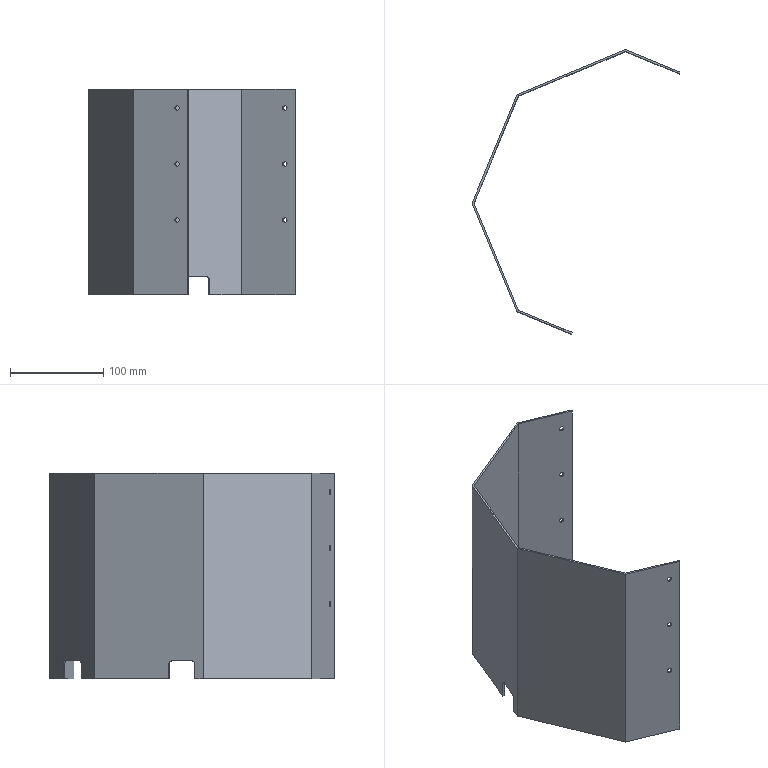Part | SolidWorks | features Cut 2, Fillet 2, ICE 2, Extrusion 1, RefAxis 1, Shell 1 | 1 solid | 38 faces | box 222.691 x 304.953 x 220 mm | volume 216770 mm3 | plane 22 | cylinder 16 | commonest cylinder face diameters 5 x12 10 x4
STEP:
#1=CARTESIAN_POINT('',(-66.179,-134.946,80.));
#2=VERTEX_POINT('',#1);
#3=CARTESIAN_POINT('',(-70.799,-133.033,80.));
#4=VERTEX_POINT('',#3);
#5=CARTESIAN_POINT('',(-68.489,-133.99,80.));
#6=DIRECTION('',(0.3827,0.9239,0.));
#7=DIRECTION('',(-0.9239,0.3827,0.));
#8=AXIS2_PLACEMENT_3D('',#5,#6,#7);
#9=CIRCLE('',#8,2.5);
#10=EDGE_CURVE('',#2,#4,#9,.T.);
#11=ORIENTED_EDGE('',*,*,#10,.T.);
#12=CARTESIAN_POINT('',(-71.564,-134.881,80.));
#13=VERTEX_POINT('',#12);
#14=CARTESIAN_POINT('',(53.29,166.544,80.));
#15=DIRECTION('',(-0.3827,-0.9239,0.));
#16=VECTOR('',#15,1000.);
#17=LINE('',#14,#16);
#18=EDGE_CURVE('',#4,#13,#17,.T.);
#19=ORIENTED_EDGE('',*,*,#18,.T.);
#20=CARTESIAN_POINT('',(-66.945,-136.794,80.));
#21=VERTEX_POINT('',#20);
#22=CARTESIAN_POINT('',(-69.254,-135.837,80.));
#23=DIRECTION('',(-0.3827,-0.9239,0.));
#24=DIRECTION('',(0.9239,-0.3827,0.));
#25=AXIS2_PLACEMENT_3D('',#22,#23,#24);
#26=CIRCLE('',#25,2.5);
#27=EDGE_CURVE('',#13,#21,#26,.T.);
#28=ORIENTED_EDGE('',*,*,#27,.T.);
#29=CARTESIAN_POINT('',(57.91,164.631,80.));
#30=DIRECTION('',(-0.3827,-0.9239,0.));
#31=VECTOR('',#30,1000.);
#32=LINE('',#29,#31);
#33=EDGE_CURVE('',#2,#21,#32,.T.);
#34=ORIENTED_EDGE('',*,*,#33,.F.);
#35=EDGE_LOOP('',(#11,#19,#28,#34));
#36=FACE_OUTER_BOUND('',#35,.T.);
#37=CARTESIAN_POINT('',(55.6,165.587,80.));
#38=DIRECTION('',(-0.3827,-0.9239,0.));
#39=DIRECTION('',(0.9239,-0.3827,0.));
#40=AXIS2_PLACEMENT_3D('',#37,#38,#39);
#41=CYLINDRICAL_SURFACE('',#40,2.5);
#42=ADVANCED_FACE('',(#36),#41,.F.);
#43=CARTESIAN_POINT('',(44.772,145.979,80.));
#44=VERTEX_POINT('',#43);
#45=CARTESIAN_POINT('',(49.391,144.065,80.));
#46=VERTEX_POINT('',#45);
#47=CARTESIAN_POINT('',(47.081,145.022,80.));
#48=DIRECTION('',(-0.3827,-0.9239,0.));
#49=DIRECTION('',(0.9239,-0.3827,0.));
#50=AXIS2_PLACEMENT_3D('',#47,#48,#49);
#51=CIRCLE('',#50,2.5);
#52=EDGE_CURVE('',#44,#46,#51,.T.);
#53=ORIENTED_EDGE('',*,*,#52,.F.);
#54=CARTESIAN_POINT('',(44.006,144.131,80.));
#55=VERTEX_POINT('',#54);
#56=CARTESIAN_POINT('',(53.29,166.544,80.));
#57=DIRECTION('',(-0.3827,-0.9239,0.));
#58=VECTOR('',#57,1000.);
#59=LINE('',#56,#58);
#60=EDGE_CURVE('',#44,#55,#59,.T.);
#61=ORIENTED_EDGE('',*,*,#60,.T.);
#62=CARTESIAN_POINT('',(48.626,142.217,80.));
#63=VERTEX_POINT('',#62);
#64=CARTESIAN_POINT('',(46.316,143.174,80.));
#65=DIRECTION('',(-0.3827,-0.9239,0.));
#66=DIRECTION('',(0.9239,-0.3827,0.));
#67=AXIS2_PLACEMENT_3D('',#64,#65,#66);
#68=CIRCLE('',#67,2.5);
#69=EDGE_CURVE('',#55,#63,#68,.T.);
#70=ORIENTED_EDGE('',*,*,#69,.T.);
#71=CARTESIAN_POINT('',(57.91,164.631,80.));
#72=DIRECTION('',(-0.3827,-0.9239,0.));
#73=VECTOR('',#72,1000.);
#74=LINE('',#71,#73);
#75=EDGE_CURVE('',#46,#63,#74,.T.);
#76=ORIENTED_EDGE('',*,*,#75,.F.);
#77=EDGE_LOOP('',(#53,#61,#70,#76));
#78=FACE_OUTER_BOUND('',#77,.T.);
#79=CARTESIAN_POINT('',(55.6,165.587,80.));
#80=DIRECTION('',(-0.3827,-0.9239,0.));
#81=DIRECTION('',(0.9239,-0.3827,0.));
#82=AXIS2_PLACEMENT_3D('',#79,#80,#81);
#83=CYLINDRICAL_SURFACE('',#82,2.5);
#84=ADVANCED_FACE('',(#78),#83,.F.);
#85=CARTESIAN_POINT('',(-66.179,-134.946,140.));
#86=VERTEX_POINT('',#85);
#87=CARTESIAN_POINT('',(-70.799,-133.033,140.));
#88=VERTEX_POINT('',#87);
#89=CARTESIAN_POINT('',(-68.489,-133.99,140.));
#90=DIRECTION('',(0.3827,0.9239,0.));
#91=DIRECTION('',(-0.9239,0.3827,0.));
#92=AXIS2_PLACEMENT_3D('',#89,#90,#91);
#93=CIRCLE('',#92,2.5);
#94=EDGE_CURVE('',#86,#88,#93,.T.);
#95=ORIENTED_EDGE('',*,*,#94,.T.);
#96=CARTESIAN_POINT('',(-71.564,-134.881,140.));
#97=VERTEX_POINT('',#96);
#98=CARTESIAN_POINT('',(53.29,166.544,140.));
#99=DIRECTION('',(-0.3827,-0.9239,0.));
#100=VECTOR('',#99,1000.);
#101=LINE('',#98,#100);
#102=EDGE_CURVE('',#88,#97,#101,.T.);
#103=ORIENTED_EDGE('',*,*,#102,.T.);
#104=CARTESIAN_POINT('',(-66.945,-136.794,140.));
#105=VERTEX_POINT('',#104);
#106=CARTESIAN_POINT('',(-69.254,-135.837,140.));
#107=DIRECTION('',(-0.3827,-0.9239,0.));
#108=DIRECTION('',(0.9239,-0.3827,0.));
#109=AXIS2_PLACEMENT_3D('',#106,#107,#108);
#110=CIRCLE('',#109,2.5);
#111=EDGE_CURVE('',#97,#105,#110,.T.);
#112=ORIENTED_EDGE('',*,*,#111,.T.);
#113=CARTESIAN_POINT('',(57.91,164.631,140.));
#114=DIRECTION('',(-0.3827,-0.9239,0.));
#115=VECTOR('',#114,1000.);
#116=LINE('',#113,#115);
#117=EDGE_CURVE('',#86,#105,#116,.T.);
#118=ORIENTED_EDGE('',*,*,#117,.F.);
#119=EDGE_LOOP('',(#95,#103,#112,#118));
#120=FACE_OUTER_BOUND('',#119,.T.);
#121=CARTESIAN_POINT('',(55.6,165.587,140.));
#122=DIRECTION('',(-0.3827,-0.9239,0.));
#123=DIRECTION('',(0.9239,-0.3827,0.));
#124=AXIS2_PLACEMENT_3D('',#121,#122,#123);
#125=CYLINDRICAL_SURFACE('',#124,2.5);
#126=ADVANCED_FACE('',(#120),#125,.F.);
#127=CARTESIAN_POINT('',(44.772,145.979,140.));
#128=VERTEX_POINT('',#127);
#129=CARTESIAN_POINT('',(49.391,144.065,140.));
#130=VERTEX_POINT('',#129);
#131=CARTESIAN_POINT('',(47.081,145.022,140.));
#132=DIRECTION('',(-0.3827,-0.9239,0.));
#133=DIRECTION('',(0.9239,-0.3827,0.));
#134=AXIS2_PLACEMENT_3D('',#131,#132,#133);
#135=CIRCLE('',#134,2.5);
#136=EDGE_CURVE('',#128,#130,#135,.T.);
#137=ORIENTED_EDGE('',*,*,#136,.F.);
#138=CARTESIAN_POINT('',(44.006,144.131,140.));
#139=VERTEX_POINT('',#138);
#140=CARTESIAN_POINT('',(53.29,166.544,140.));
#141=DIRECTION('',(-0.3827,-0.9239,0.));
#142=VECTOR('',#141,1000.);
#143=LINE('',#140,#142);
#144=EDGE_CURVE('',#128,#139,#143,.T.);
#145=ORIENTED_EDGE('',*,*,#144,.T.);
#146=CARTESIAN_POINT('',(48.626,142.217,140.));
#147=VERTEX_POINT('',#146);
#148=CARTESIAN_POINT('',(46.316,143.174,140.));
#149=DIRECTION('',(-0.3827,-0.9239,0.));
#150=DIRECTION('',(0.9239,-0.3827,0.));
#151=AXIS2_PLACEMENT_3D('',#148,#149,#150);
#152=CIRCLE('',#151,2.5);
#153=EDGE_CURVE('',#139,#147,#152,.T.);
#154=ORIENTED_EDGE('',*,*,#153,.T.);
#155=CARTESIAN_POINT('',(57.91,164.631,140.));
#156=DIRECTION('',(-0.3827,-0.9239,0.));
#157=VECTOR('',#156,1000.);
#158=LINE('',#155,#157);
#159=EDGE_CURVE('',#130,#147,#158,.T.);
#160=ORIENTED_EDGE('',*,*,#159,.F.);
#161=EDGE_LOOP('',(#137,#145,#154,#160));
#162=FACE_OUTER_BOUND('',#161,.T.);
#163=CARTESIAN_POINT('',(55.6,165.587,140.));
#164=DIRECTION('',(-0.3827,-0.9239,0.));
#165=DIRECTION('',(0.9239,-0.3827,0.));
#166=AXIS2_PLACEMENT_3D('',#163,#164,#165);
#167=CYLINDRICAL_SURFACE('',#166,2.5);
#168=ADVANCED_FACE('',(#162),#167,.F.);
#169=CARTESIAN_POINT('',(-66.179,-134.946,200.));
#170=VERTEX_POINT('',#169);
#171=CARTESIAN_POINT('',(-70.799,-133.033,200.));
#172=VERTEX_POINT('',#171);
#173=CARTESIAN_POINT('',(-68.489,-133.99,200.));
#174=DIRECTION('',(0.3827,0.9239,0.));
#175=DIRECTION('',(-0.9239,0.3827,0.));
#176=AXIS2_PLACEMENT_3D('',#173,#174,#175);
#177=CIRCLE('',#176,2.5);
#178=EDGE_CURVE('',#170,#172,#177,.T.);
#179=ORIENTED_EDGE('',*,*,#178,.T.);
#180=CARTESIAN_POINT('',(-71.564,-134.881,200.));
#181=VERTEX_POINT('',#180);
#182=CARTESIAN_POINT('',(53.29,166.544,200.));
#183=DIRECTION('',(-0.3827,-0.9239,0.));
#184=VECTOR('',#183,1000.);
#185=LINE('',#182,#184);
#186=EDGE_CURVE('',#172,#181,#185,.T.);
#187=ORIENTED_EDGE('',*,*,#186,.T.);
#188=CARTESIAN_POINT('',(-66.945,-136.794,200.));
#189=VERTEX_POINT('',#188);
#190=CARTESIAN_POINT('',(-69.254,-135.837,200.));
#191=DIRECTION('',(-0.3827,-0.9239,0.));
#192=DIRECTION('',(0.9239,-0.3827,0.));
#193=AXIS2_PLACEMENT_3D('',#190,#191,#192);
#194=CIRCLE('',#193,2.5);
#195=EDGE_CURVE('',#181,#189,#194,.T.);
#196=ORIENTED_EDGE('',*,*,#195,.T.);
#197=CARTESIAN_POINT('',(57.91,164.631,200.));
#198=DIRECTION('',(-0.3827,-0.9239,0.));
#199=VECTOR('',#198,1000.);
#200=LINE('',#197,#199);
#201=EDGE_CURVE('',#170,#189,#200,.T.);
#202=ORIENTED_EDGE('',*,*,#201,.F.);
#203=EDGE_LOOP('',(#179,#187,#196,#202));
#204=FACE_OUTER_BOUND('',#203,.T.);
#205=CARTESIAN_POINT('',(55.6,165.587,200.));
#206=DIRECTION('',(-0.3827,-0.9239,0.));
#207=DIRECTION('',(0.9239,-0.3827,0.));
#208=AXIS2_PLACEMENT_3D('',#205,#206,#207);
#209=CYLINDRICAL_SURFACE('',#208,2.5);
#210=ADVANCED_FACE('',(#204),#209,.F.);
#211=CARTESIAN_POINT('',(44.772,145.979,200.));
#212=VERTEX_POINT('',#211);
#213=CARTESIAN_POINT('',(49.391,144.065,200.));
#214=VERTEX_POINT('',#213);
#215=CARTESIAN_POINT('',(47.081,145.022,200.));
#216=DIRECTION('',(-0.3827,-0.9239,0.));
#217=DIRECTION('',(0.9239,-0.3827,0.));
#218=AXIS2_PLACEMENT_3D('',#215,#216,#217);
#219=CIRCLE('',#218,2.5);
#220=EDGE_CURVE('',#212,#214,#219,.T.);
#221=ORIENTED_EDGE('',*,*,#220,.F.);
#222=CARTESIAN_POINT('',(44.006,144.131,200.));
#223=VERTEX_POINT('',#222);
#224=CARTESIAN_POINT('',(53.29,166.544,200.));
#225=DIRECTION('',(-0.3827,-0.9239,0.));
#226=VECTOR('',#225,1000.);
#227=LINE('',#224,#226);
#228=EDGE_CURVE('',#212,#223,#227,.T.);
#229=ORIENTED_EDGE('',*,*,#228,.T.);
#230=CARTESIAN_POINT('',(48.626,142.217,200.));
#231=VERTEX_POINT('',#230);
#232=CARTESIAN_POINT('',(46.316,143.174,200.));
#233=DIRECTION('',(-0.3827,-0.9239,0.));
#234=DIRECTION('',(0.9239,-0.3827,0.));
#235=AXIS2_PLACEMENT_3D('',#232,#233,#234);
#236=CIRCLE('',#235,2.5);
#237=EDGE_CURVE('',#223,#231,#236,.T.);
#238=ORIENTED_EDGE('',*,*,#237,.T.);
#239=CARTESIAN_POINT('',(57.91,164.631,200.));
#240=DIRECTION('',(-0.3827,-0.9239,0.));
#241=VECTOR('',#240,1000.);
#242=LINE('',#239,#241);
#243=EDGE_CURVE('',#214,#231,#242,.T.);
#244=ORIENTED_EDGE('',*,*,#243,.F.);
#245=EDGE_LOOP('',(#221,#229,#238,#244));
#246=FACE_OUTER_BOUND('',#245,.T.);
#247=CARTESIAN_POINT('',(55.6,165.587,200.));
#248=DIRECTION('',(-0.3827,-0.9239,0.));
#249=DIRECTION('',(0.9239,-0.3827,0.));
#250=AXIS2_PLACEMENT_3D('',#247,#248,#249);
#251=CYLINDRICAL_SURFACE('',#250,2.5);
#252=ADVANCED_FACE('',(#246),#251,.F.);
#253=CARTESIAN_POINT('',(0.,162.359,0.));
#254=VERTEX_POINT('',#253);
#255=CARTESIAN_POINT('',(-34.269,148.164,0.));
#256=VERTEX_POINT('',#255);
#257=CARTESIAN_POINT('',(0.7654,162.676,0.));
#258=DIRECTION('',(-0.9239,-0.3827,0.));
#259=VECTOR('',#258,1000.);
#260=LINE('',#257,#259);
#261=EDGE_CURVE('',#254,#256,#260,.T.);
#262=ORIENTED_EDGE('',*,*,#261,.T.);
#263=CARTESIAN_POINT('',(-35.034,150.012,0.));
#264=VERTEX_POINT('',#263);
#265=CARTESIAN_POINT('',(81.301,-130.847,0.));
#266=DIRECTION('',(-0.3827,0.9239,0.));
#267=VECTOR('',#266,1000.);
#268=LINE('',#265,#267);
#269=EDGE_CURVE('',#256,#264,#268,.T.);
#270=ORIENTED_EDGE('',*,*,#269,.T.);
#271=CARTESIAN_POINT('',(0.,164.524,0.));
#272=VERTEX_POINT('',#271);
#273=CARTESIAN_POINT('',(0.,164.524,0.));
#274=DIRECTION('',(-0.9239,-0.3827,0.));
#275=VECTOR('',#274,1000.);
#276=LINE('',#273,#275);
#277=EDGE_CURVE('',#272,#264,#276,.T.);
#278=ORIENTED_EDGE('',*,*,#277,.F.);
#279=CARTESIAN_POINT('',(58.168,140.43,0.));
#280=VERTEX_POINT('',#279);
#281=CARTESIAN_POINT('',(116.336,116.336,0.));
#282=DIRECTION('',(-0.9239,0.3827,0.));
#283=VECTOR('',#282,1000.);
#284=LINE('',#281,#283);
#285=EDGE_CURVE('',#280,#272,#284,.T.);
#286=ORIENTED_EDGE('',*,*,#285,.F.);
#287=CARTESIAN_POINT('',(57.403,138.582,0.));
#288=VERTEX_POINT('',#287);
#289=CARTESIAN_POINT('',(75.617,182.555,0.));
#290=DIRECTION('',(-0.3827,-0.9239,0.));
#291=VECTOR('',#290,1000.);
#292=LINE('',#289,#291);
#293=EDGE_CURVE('',#280,#288,#292,.T.);
#294=ORIENTED_EDGE('',*,*,#293,.T.);
#295=CARTESIAN_POINT('',(115.57,114.488,0.));
#296=DIRECTION('',(-0.9239,0.3827,0.));
#297=VECTOR('',#296,1000.);
#298=LINE('',#295,#297);
#299=EDGE_CURVE('',#288,#254,#298,.T.);
#300=ORIENTED_EDGE('',*,*,#299,.T.);
#301=EDGE_LOOP('',(#262,#270,#278,#286,#294,#300));
#302=FACE_OUTER_BOUND('',#301,.T.);
#303=CARTESIAN_POINT('',(0.,0.,0.));
#304=DIRECTION('',(0.,0.,1.));
#305=DIRECTION('',(1.,0.,0.));
#306=AXIS2_PLACEMENT_3D('',#303,#304,#305);
#307=PLANE('',#306);
#308=ADVANCED_FACE('',(#302),#307,.F.);
#309=CARTESIAN_POINT('',(-81.228,130.878,0.));
#310=VERTEX_POINT('',#309);
#311=CARTESIAN_POINT('',(-116.336,116.336,0.));
#312=VERTEX_POINT('',#311);
#313=CARTESIAN_POINT('',(0.,164.524,0.));
#314=DIRECTION('',(-0.9239,-0.3827,0.));
#315=VECTOR('',#314,1000.);
#316=LINE('',#313,#315);
#317=EDGE_CURVE('',#310,#312,#316,.T.);
#318=ORIENTED_EDGE('',*,*,#317,.F.);
#319=CARTESIAN_POINT('',(-80.463,129.03,0.));
#320=VERTEX_POINT('',#319);
#321=CARTESIAN_POINT('',(35.107,-149.982,0.));
#322=DIRECTION('',(-0.3827,0.9239,0.));
#323=VECTOR('',#322,1000.);
#324=LINE('',#321,#323);
#325=EDGE_CURVE('',#320,#310,#324,.T.);
#326=ORIENTED_EDGE('',*,*,#325,.F.);
#327=CARTESIAN_POINT('',(-114.805,114.805,0.));
#328=VERTEX_POINT('',#327);
#329=CARTESIAN_POINT('',(0.7654,162.676,0.));
#330=DIRECTION('',(-0.9239,-0.3827,0.));
#331=VECTOR('',#330,1000.);
#332=LINE('',#329,#331);
#333=EDGE_CURVE('',#320,#328,#332,.T.);
#334=ORIENTED_EDGE('',*,*,#333,.T.);
#335=CARTESIAN_POINT('',(-147.369,36.19,0.));
#336=VERTEX_POINT('',#335);
#337=CARTESIAN_POINT('',(-114.488,115.57,0.));
#338=DIRECTION('',(-0.3827,-0.9239,0.));
#339=VECTOR('',#338,1000.);
#340=LINE('',#337,#339);
#341=EDGE_CURVE('',#328,#336,#340,.T.);
#342=ORIENTED_EDGE('',*,*,#341,.T.);
#343=CARTESIAN_POINT('',(-149.216,36.955,0.));
#344=VERTEX_POINT('',#343);
#345=CARTESIAN_POINT('',(90.512,-62.344,0.));
#346=DIRECTION('',(-0.9239,0.3827,0.));
#347=VECTOR('',#346,1000.);
#348=LINE('',#345,#347);
#349=EDGE_CURVE('',#336,#344,#348,.T.);
#350=ORIENTED_EDGE('',*,*,#349,.T.);
#351=CARTESIAN_POINT('',(-116.336,116.336,0.));
#352=DIRECTION('',(-0.3827,-0.9239,0.));
#353=VECTOR('',#352,1000.);
#354=LINE('',#351,#353);
#355=EDGE_CURVE('',#312,#344,#354,.T.);
#356=ORIENTED_EDGE('',*,*,#355,.F.);
#357=EDGE_LOOP('',(#318,#326,#334,#342,#350,#356));
#358=FACE_OUTER_BOUND('',#357,.T.);
#359=CARTESIAN_POINT('',(0.,0.,0.));
#360=DIRECTION('',(0.,0.,1.));
#361=DIRECTION('',(1.,0.,0.));
#362=AXIS2_PLACEMENT_3D('',#359,#360,#361);
#363=PLANE('',#362);
#364=ADVANCED_FACE('',(#358),#363,.F.);
#365=CARTESIAN_POINT('',(-69.254,-135.837,80.));
#366=DIRECTION('',(-0.3827,-0.9239,0.));
#367=DIRECTION('',(0.9239,-0.3827,0.));
#368=AXIS2_PLACEMENT_3D('',#365,#366,#367);
#369=CIRCLE('',#368,2.5);
#370=EDGE_CURVE('',#21,#13,#369,.T.);
#371=ORIENTED_EDGE('',*,*,#370,.F.);
#372=ORIENTED_EDGE('',*,*,#27,.F.);
#373=EDGE_LOOP('',(#371,#372));
#374=FACE_BOUND('',#373,.T.);
#375=CARTESIAN_POINT('',(-69.254,-135.837,140.));
#376=DIRECTION('',(-0.3827,-0.9239,0.));
#377=DIRECTION('',(0.9239,-0.3827,0.));
#378=AXIS2_PLACEMENT_3D('',#375,#376,#377);
#379=CIRCLE('',#378,2.5);
#380=EDGE_CURVE('',#105,#97,#379,.T.);
#381=ORIENTED_EDGE('',*,*,#380,.F.);
#382=ORIENTED_EDGE('',*,*,#111,.F.);
#383=EDGE_LOOP('',(#381,#382));
#384=FACE_BOUND('',#383,.T.);
#385=CARTESIAN_POINT('',(-69.254,-135.837,200.));
#386=DIRECTION('',(-0.3827,-0.9239,0.));
#387=DIRECTION('',(0.9239,-0.3827,0.));
#388=AXIS2_PLACEMENT_3D('',#385,#386,#387);
#389=CIRCLE('',#388,2.5);
#390=EDGE_CURVE('',#189,#181,#389,.T.);
#391=ORIENTED_EDGE('',*,*,#390,.F.);
#392=ORIENTED_EDGE('',*,*,#195,.F.);
#393=EDGE_LOOP('',(#391,#392));
#394=FACE_BOUND('',#393,.T.);
#395=CARTESIAN_POINT('',(-116.336,-116.336,0.));
#396=VERTEX_POINT('',#395);
#397=CARTESIAN_POINT('',(-58.168,-140.43,0.));
#398=VERTEX_POINT('',#397);
#399=CARTESIAN_POINT('',(-116.336,-116.336,0.));
#400=DIRECTION('',(0.9239,-0.3827,0.));
#401=VECTOR('',#400,1000.);
#402=LINE('',#399,#401);
#403=EDGE_CURVE('',#396,#398,#402,.T.);
#404=ORIENTED_EDGE('',*,*,#403,.T.);
#405=CARTESIAN_POINT('',(-58.168,-140.43,220.));
#406=VERTEX_POINT('',#405);
#407=CARTESIAN_POINT('',(-58.168,-140.43,220.));
#408=DIRECTION('',(0.,0.,1.));
#409=VECTOR('',#408,1000.);
#410=LINE('',#407,#409);
#411=EDGE_CURVE('',#398,#406,#410,.T.);
#412=ORIENTED_EDGE('',*,*,#411,.T.);
#413=CARTESIAN_POINT('',(-116.336,-116.336,220.));
#414=VERTEX_POINT('',#413);
#415=CARTESIAN_POINT('',(-116.336,-116.336,220.));
#416=DIRECTION('',(0.9239,-0.3827,0.));
#417=VECTOR('',#416,1000.);
#418=LINE('',#415,#417);
#419=EDGE_CURVE('',#414,#406,#418,.T.);
#420=ORIENTED_EDGE('',*,*,#419,.F.);
#421=CARTESIAN_POINT('',(-116.336,-116.336,220.));
#422=DIRECTION('',(0.,0.,-1.));
#423=VECTOR('',#422,1000.);
#424=LINE('',#421,#423);
#425=EDGE_CURVE('',#414,#396,#424,.T.);
#426=ORIENTED_EDGE('',*,*,#425,.T.);
#427=EDGE_LOOP('',(#404,#412,#420,#426));
#428=FACE_OUTER_BOUND('',#427,.T.);
#429=CARTESIAN_POINT('',(-116.336,-116.336,220.));
#430=DIRECTION('',(0.3827,0.9239,0.));
#431=DIRECTION('',(-0.9239,0.3827,0.));
#432=AXIS2_PLACEMENT_3D('',#429,#430,#431);
#433=PLANE('',#432);
#434=ADVANCED_FACE('',(#374,#384,#394,#428),#433,.F.);
#435=CARTESIAN_POINT('',(47.081,145.022,80.));
#436=DIRECTION('',(-0.3827,-0.9239,0.));
#437=DIRECTION('',(0.9239,-0.3827,0.));
#438=AXIS2_PLACEMENT_3D('',#435,#436,#437);
#439=CIRCLE('',#438,2.5);
#440=EDGE_CURVE('',#46,#44,#439,.T.);
#441=ORIENTED_EDGE('',*,*,#440,.T.);
#442=ORIENTED_EDGE('',*,*,#52,.T.);
#443=EDGE_LOOP('',(#441,#442));
#444=FACE_BOUND('',#443,.T.);
#445=CARTESIAN_POINT('',(47.081,145.022,140.));
#446=DIRECTION('',(-0.3827,-0.9239,0.));
#447=DIRECTION('',(0.9239,-0.3827,0.));
#448=AXIS2_PLACEMENT_3D('',#445,#446,#447);
#449=CIRCLE('',#448,2.5);
#450=EDGE_CURVE('',#130,#128,#449,.T.);
#451=ORIENTED_EDGE('',*,*,#450,.T.);
#452=ORIENTED_EDGE('',*,*,#136,.T.);
#453=EDGE_LOOP('',(#451,#452));
#454=FACE_BOUND('',#453,.T.);
#455=CARTESIAN_POINT('',(47.081,145.022,200.));
#456=DIRECTION('',(-0.3827,-0.9239,0.));
#457=DIRECTION('',(0.9239,-0.3827,0.));
#458=AXIS2_PLACEMENT_3D('',#455,#456,#457);
#459=CIRCLE('',#458,2.5);
#460=EDGE_CURVE('',#214,#212,#459,.T.);
#461=ORIENTED_EDGE('',*,*,#460,.T.);
#462=ORIENTED_EDGE('',*,*,#220,.T.);
#463=EDGE_LOOP('',(#461,#462));
#464=FACE_BOUND('',#463,.T.);
#465=CARTESIAN_POINT('',(58.168,140.43,220.));
#466=VERTEX_POINT('',#465);
#467=CARTESIAN_POINT('',(0.,164.524,220.));
#468=VERTEX_POINT('',#467);
#469=CARTESIAN_POINT('',(116.336,116.336,220.));
#470=DIRECTION('',(-0.9239,0.3827,0.));
#471=VECTOR('',#470,1000.);
#472=LINE('',#469,#471);
#473=EDGE_CURVE('',#466,#468,#472,.T.);
#474=ORIENTED_EDGE('',*,*,#473,.F.);
#475=CARTESIAN_POINT('',(58.168,140.43,220.));
#476=DIRECTION('',(0.,0.,-1.));
#477=VECTOR('',#476,1000.);
#478=LINE('',#475,#477);
#479=EDGE_CURVE('',#466,#280,#478,.T.);
#480=ORIENTED_EDGE('',*,*,#479,.T.);
#481=ORIENTED_EDGE('',*,*,#285,.T.);
#482=CARTESIAN_POINT('',(0.,164.524,220.));
#483=DIRECTION('',(0.,0.,-1.));
#484=VECTOR('',#483,1000.);
#485=LINE('',#482,#484);
#486=EDGE_CURVE('',#468,#272,#485,.T.);
#487=ORIENTED_EDGE('',*,*,#486,.F.);
#488=EDGE_LOOP('',(#474,#480,#481,#487));
#489=FACE_OUTER_BOUND('',#488,.T.);
#490=CARTESIAN_POINT('',(116.336,116.336,220.));
#491=DIRECTION('',(-0.3827,-0.9239,0.));
#492=DIRECTION('',(0.9239,-0.3827,0.));
#493=AXIS2_PLACEMENT_3D('',#490,#491,#492);
#494=PLANE('',#493);
#495=ADVANCED_FACE('',(#444,#454,#464,#489),#494,.F.);
#496=ORIENTED_EDGE('',*,*,#277,.T.);
#497=CARTESIAN_POINT('',(-35.034,150.012,15.));
#498=VERTEX_POINT('',#497);
#499=CARTESIAN_POINT('',(-35.034,150.012,0.));
#500=DIRECTION('',(0.,0.,-1.));
#501=VECTOR('',#500,1000.);
#502=LINE('',#499,#501);
#503=EDGE_CURVE('',#498,#264,#502,.T.);
#504=ORIENTED_EDGE('',*,*,#503,.F.);
#505=CARTESIAN_POINT('',(-39.654,148.098,20.));
#506=VERTEX_POINT('',#505);
#507=CARTESIAN_POINT('',(-39.654,148.098,15.));
#508=DIRECTION('',(0.3827,-0.9239,0.));
#509=DIRECTION('',(0.9239,0.3827,0.));
#510=AXIS2_PLACEMENT_3D('',#507,#508,#509);
#511=CIRCLE('',#510,5.);
#512=EDGE_CURVE('',#498,#506,#511,.T.);
#513=ORIENTED_EDGE('',*,*,#512,.T.);
#514=CARTESIAN_POINT('',(-76.609,132.791,20.));
#515=VERTEX_POINT('',#514);
#516=CARTESIAN_POINT('',(-35.034,150.012,20.));
#517=DIRECTION('',(0.9239,0.3827,0.));
#518=VECTOR('',#517,1000.);
#519=LINE('',#516,#518);
#520=EDGE_CURVE('',#515,#506,#519,.T.);
#521=ORIENTED_EDGE('',*,*,#520,.F.);
#522=CARTESIAN_POINT('',(-81.228,130.878,15.));
#523=VERTEX_POINT('',#522);
#524=CARTESIAN_POINT('',(-76.609,132.791,15.));
#525=DIRECTION('',(0.3827,-0.9239,0.));
#526=DIRECTION('',(0.9239,0.3827,0.));
#527=AXIS2_PLACEMENT_3D('',#524,#525,#526);
#528=CIRCLE('',#527,5.);
#529=EDGE_CURVE('',#515,#523,#528,.T.);
#530=ORIENTED_EDGE('',*,*,#529,.T.);
#531=CARTESIAN_POINT('',(-81.228,130.878,0.));
#532=DIRECTION('',(0.,0.,1.));
#533=VECTOR('',#532,1000.);
#534=LINE('',#531,#533);
#535=EDGE_CURVE('',#310,#523,#534,.T.);
#536=ORIENTED_EDGE('',*,*,#535,.F.);
#537=ORIENTED_EDGE('',*,*,#317,.T.);
#538=CARTESIAN_POINT('',(-116.336,116.336,220.));
#539=VERTEX_POINT('',#538);
#540=CARTESIAN_POINT('',(-116.336,116.336,220.));
#541=DIRECTION('',(0.,0.,-1.));
#542=VECTOR('',#541,1000.);
#543=LINE('',#540,#542);
#544=EDGE_CURVE('',#539,#312,#543,.T.);
#545=ORIENTED_EDGE('',*,*,#544,.F.);
#546=CARTESIAN_POINT('',(0.,164.524,220.));
#547=DIRECTION('',(-0.9239,-0.3827,0.));
#548=VECTOR('',#547,1000.);
#549=LINE('',#546,#548);
#550=EDGE_CURVE('',#468,#539,#549,.T.);
#551=ORIENTED_EDGE('',*,*,#550,.F.);
#552=ORIENTED_EDGE('',*,*,#486,.T.);
#553=EDGE_LOOP('',(#496,#504,#513,#521,#530,#536,#537,#545,#551,#552));
#554=FACE_OUTER_BOUND('',#553,.T.);
#555=CARTESIAN_POINT('',(0.,164.524,220.));
#556=DIRECTION('',(0.3827,-0.9239,0.));
#557=DIRECTION('',(0.9239,0.3827,0.));
#558=AXIS2_PLACEMENT_3D('',#555,#556,#557);
#559=PLANE('',#558);
#560=ADVANCED_FACE('',(#554),#559,.F.);
#561=ORIENTED_EDGE('',*,*,#355,.T.);
#562=CARTESIAN_POINT('',(-149.216,36.955,15.));
#563=VERTEX_POINT('',#562);
#564=CARTESIAN_POINT('',(-149.216,36.955,0.));
#565=DIRECTION('',(0.,0.,-1.));
#566=VECTOR('',#565,1000.);
#567=LINE('',#564,#566);
#568=EDGE_CURVE('',#563,#344,#567,.T.);
#569=ORIENTED_EDGE('',*,*,#568,.F.);
#570=CARTESIAN_POINT('',(-151.13,32.336,20.));
#571=VERTEX_POINT('',#570);
#572=CARTESIAN_POINT('',(-151.13,32.336,15.));
#573=DIRECTION('',(0.9239,-0.3827,0.));
#574=DIRECTION('',(0.3827,0.9239,0.));
#575=AXIS2_PLACEMENT_3D('',#572,#573,#574);
#576=CIRCLE('',#575,5.);
#577=EDGE_CURVE('',#563,#571,#576,.T.);
#578=ORIENTED_EDGE('',*,*,#577,.T.);
#579=CARTESIAN_POINT('',(-158.783,13.858,20.));
#580=VERTEX_POINT('',#579);
#581=CARTESIAN_POINT('',(-149.216,36.955,20.));
#582=DIRECTION('',(0.3827,0.9239,0.));
#583=VECTOR('',#582,1000.);
#584=LINE('',#581,#583);
#585=EDGE_CURVE('',#580,#571,#584,.T.);
#586=ORIENTED_EDGE('',*,*,#585,.F.);
#587=CARTESIAN_POINT('',(-160.697,9.239,15.));
#588=VERTEX_POINT('',#587);
#589=CARTESIAN_POINT('',(-158.783,13.858,15.));
#590=DIRECTION('',(0.9239,-0.3827,0.));
#591=DIRECTION('',(0.3827,0.9239,0.));
#592=AXIS2_PLACEMENT_3D('',#589,#590,#591);
#593=CIRCLE('',#592,5.);
#594=EDGE_CURVE('',#580,#588,#593,.T.);
#595=ORIENTED_EDGE('',*,*,#594,.T.);
#596=CARTESIAN_POINT('',(-160.697,9.239,0.));
#597=VERTEX_POINT('',#596);
#598=CARTESIAN_POINT('',(-160.697,9.239,0.));
#599=DIRECTION('',(0.,0.,1.));
#600=VECTOR('',#599,1000.);
#601=LINE('',#598,#600);
#602=EDGE_CURVE('',#597,#588,#601,.T.);
#603=ORIENTED_EDGE('',*,*,#602,.F.);
#604=CARTESIAN_POINT('',(-164.524,0.,0.));
#605=VERTEX_POINT('',#604);
#606=CARTESIAN_POINT('',(-116.336,116.336,0.));
#607=DIRECTION('',(-0.3827,-0.9239,0.));
#608=VECTOR('',#607,1000.);
#609=LINE('',#606,#608);
#610=EDGE_CURVE('',#597,#605,#609,.T.);
#611=ORIENTED_EDGE('',*,*,#610,.T.);
#612=CARTESIAN_POINT('',(-164.524,0.,220.));
#613=VERTEX_POINT('',#612);
#614=CARTESIAN_POINT('',(-164.524,0.,220.));
#615=DIRECTION('',(0.,0.,-1.));
#616=VECTOR('',#615,1000.);
#617=LINE('',#614,#616);
#618=EDGE_CURVE('',#613,#605,#617,.T.);
#619=ORIENTED_EDGE('',*,*,#618,.F.);
#620=CARTESIAN_POINT('',(-116.336,116.336,220.));
#621=DIRECTION('',(-0.3827,-0.9239,0.));
#622=VECTOR('',#621,1000.);
#623=LINE('',#620,#622);
#624=EDGE_CURVE('',#539,#613,#623,.T.);
#625=ORIENTED_EDGE('',*,*,#624,.F.);
#626=ORIENTED_EDGE('',*,*,#544,.T.);
#627=EDGE_LOOP('',(#561,#569,#578,#586,#595,#603,#611,#619,#625,#626));
#628=FACE_OUTER_BOUND('',#627,.T.);
#629=CARTESIAN_POINT('',(-116.336,116.336,220.));
#630=DIRECTION('',(0.9239,-0.3827,0.));
#631=DIRECTION('',(0.3827,0.9239,0.));
#632=AXIS2_PLACEMENT_3D('',#629,#630,#631);
#633=PLANE('',#632);
#634=ADVANCED_FACE('',(#628),#633,.F.);
#635=CARTESIAN_POINT('',(-164.524,0.,0.));
#636=DIRECTION('',(0.3827,-0.9239,0.));
#637=VECTOR('',#636,1000.);
#638=LINE('',#635,#637);
#639=EDGE_CURVE('',#605,#396,#638,.T.);
#640=ORIENTED_EDGE('',*,*,#639,.T.);
#641=ORIENTED_EDGE('',*,*,#425,.F.);
#642=CARTESIAN_POINT('',(-164.524,0.,220.));
#643=DIRECTION('',(0.3827,-0.9239,0.));
#644=VECTOR('',#643,1000.);
#645=LINE('',#642,#644);
#646=EDGE_CURVE('',#613,#414,#645,.T.);
#647=ORIENTED_EDGE('',*,*,#646,.F.);
#648=ORIENTED_EDGE('',*,*,#618,.T.);
#649=EDGE_LOOP('',(#640,#641,#647,#648));
#650=FACE_OUTER_BOUND('',#649,.T.);
#651=CARTESIAN_POINT('',(-164.524,0.,220.));
#652=DIRECTION('',(0.9239,0.3827,0.));
#653=DIRECTION('',(-0.3827,0.9239,0.));
#654=AXIS2_PLACEMENT_3D('',#651,#652,#653);
#655=PLANE('',#654);
#656=ADVANCED_FACE('',(#650),#655,.F.);
#657=CARTESIAN_POINT('',(57.403,138.582,220.));
#658=VERTEX_POINT('',#657);
#659=CARTESIAN_POINT('',(75.617,182.555,220.));
#660=DIRECTION('',(-0.3827,-0.9239,0.));
#661=VECTOR('',#660,1000.);
#662=LINE('',#659,#661);
#663=EDGE_CURVE('',#466,#658,#662,.T.);
#664=ORIENTED_EDGE('',*,*,#663,.F.);
#665=ORIENTED_EDGE('',*,*,#473,.T.);
#666=ORIENTED_EDGE('',*,*,#550,.T.);
#667=ORIENTED_EDGE('',*,*,#624,.T.);
#668=ORIENTED_EDGE('',*,*,#646,.T.);
#669=ORIENTED_EDGE('',*,*,#419,.T.);
#670=CARTESIAN_POINT('',(-57.403,-138.582,220.));
#671=VERTEX_POINT('',#670);
#672=CARTESIAN_POINT('',(75.617,182.555,220.));
#673=DIRECTION('',(-0.3827,-0.9239,0.));
#674=VECTOR('',#673,1000.);
#675=LINE('',#672,#674);
#676=EDGE_CURVE('',#671,#406,#675,.T.);
#677=ORIENTED_EDGE('',*,*,#676,.F.);
#678=CARTESIAN_POINT('',(-114.805,-114.805,220.));
#679=VERTEX_POINT('',#678);
#680=CARTESIAN_POINT('',(-115.57,-114.488,220.));
#681=DIRECTION('',(0.9239,-0.3827,0.));
#682=VECTOR('',#681,1000.);
#683=LINE('',#680,#682);
#684=EDGE_CURVE('',#679,#671,#683,.T.);
#685=ORIENTED_EDGE('',*,*,#684,.F.);
#686=CARTESIAN_POINT('',(-162.359,0.,220.));
#687=VERTEX_POINT('',#686);
#688=CARTESIAN_POINT('',(-162.676,0.7654,220.));
#689=DIRECTION('',(0.3827,-0.9239,0.));
#690=VECTOR('',#689,1000.);
#691=LINE('',#688,#690);
#692=EDGE_CURVE('',#687,#679,#691,.T.);
#693=ORIENTED_EDGE('',*,*,#692,.F.);
#694=CARTESIAN_POINT('',(-114.805,114.805,220.));
#695=VERTEX_POINT('',#694);
#696=CARTESIAN_POINT('',(-114.488,115.57,220.));
#697=DIRECTION('',(-0.3827,-0.9239,0.));
#698=VECTOR('',#697,1000.);
#699=LINE('',#696,#698);
#700=EDGE_CURVE('',#695,#687,#699,.T.);
#701=ORIENTED_EDGE('',*,*,#700,.F.);
#702=CARTESIAN_POINT('',(0.,162.359,220.));
#703=VERTEX_POINT('',#702);
#704=CARTESIAN_POINT('',(0.7654,162.676,220.));
#705=DIRECTION('',(-0.9239,-0.3827,0.));
#706=VECTOR('',#705,1000.);
#707=LINE('',#704,#706);
#708=EDGE_CURVE('',#703,#695,#707,.T.);
#709=ORIENTED_EDGE('',*,*,#708,.F.);
#710=CARTESIAN_POINT('',(115.57,114.488,220.));
#711=DIRECTION('',(-0.9239,0.3827,0.));
#712=VECTOR('',#711,1000.);
#713=LINE('',#710,#712);
#714=EDGE_CURVE('',#658,#703,#713,.T.);
#715=ORIENTED_EDGE('',*,*,#714,.F.);
#716=EDGE_LOOP('',(#664,#665,#666,#667,#668,#669,#677,#685,#693,#701,#709,#715));
#717=FACE_OUTER_BOUND('',#716,.T.);
#718=CARTESIAN_POINT('',(0.,0.,220.));
#719=DIRECTION('',(0.,0.,1.));
#720=DIRECTION('',(1.,0.,0.));
#721=AXIS2_PLACEMENT_3D('',#718,#719,#720);
#722=PLANE('',#721);
#723=ADVANCED_FACE('',(#717),#722,.T.);
#724=ORIENTED_EDGE('',*,*,#610,.F.);
#725=CARTESIAN_POINT('',(-158.849,8.473,0.));
#726=VERTEX_POINT('',#725);
#727=CARTESIAN_POINT('',(79.032,-90.06,0.));
#728=DIRECTION('',(-0.9239,0.3827,0.));
#729=VECTOR('',#728,1000.);
#730=LINE('',#727,#729);
#731=EDGE_CURVE('',#726,#597,#730,.T.);
#732=ORIENTED_EDGE('',*,*,#731,.F.);
#733=CARTESIAN_POINT('',(-162.359,0.,0.));
#734=VERTEX_POINT('',#733);
#735=CARTESIAN_POINT('',(-114.488,115.57,0.));
#736=DIRECTION('',(-0.3827,-0.9239,0.));
#737=VECTOR('',#736,1000.);
#738=LINE('',#735,#737);
#739=EDGE_CURVE('',#726,#734,#738,.T.);
#740=ORIENTED_EDGE('',*,*,#739,.T.);
#741=CARTESIAN_POINT('',(-114.805,-114.805,0.));
#742=VERTEX_POINT('',#741);
#743=CARTESIAN_POINT('',(-162.676,0.7654,0.));
#744=DIRECTION('',(0.3827,-0.9239,0.));
#745=VECTOR('',#744,1000.);
#746=LINE('',#743,#745);
#747=EDGE_CURVE('',#734,#742,#746,.T.);
#748=ORIENTED_EDGE('',*,*,#747,.T.);
#749=CARTESIAN_POINT('',(-57.403,-138.582,0.));
#750=VERTEX_POINT('',#749);
#751=CARTESIAN_POINT('',(-115.57,-114.488,0.));
#752=DIRECTION('',(0.9239,-0.3827,0.));
#753=VECTOR('',#752,1000.);
#754=LINE('',#751,#753);
#755=EDGE_CURVE('',#742,#750,#754,.T.);
#756=ORIENTED_EDGE('',*,*,#755,.T.);
#757=CARTESIAN_POINT('',(75.617,182.555,0.));
#758=DIRECTION('',(-0.3827,-0.9239,0.));
#759=VECTOR('',#758,1000.);
#760=LINE('',#757,#759);
#761=EDGE_CURVE('',#750,#398,#760,.T.);
#762=ORIENTED_EDGE('',*,*,#761,.T.);
#763=ORIENTED_EDGE('',*,*,#403,.F.);
#764=ORIENTED_EDGE('',*,*,#639,.F.);
#765=EDGE_LOOP('',(#724,#732,#740,#748,#756,#762,#763,#764));
#766=FACE_OUTER_BOUND('',#765,.T.);
#767=CARTESIAN_POINT('',(0.,0.,0.));
#768=DIRECTION('',(0.,0.,1.));
#769=DIRECTION('',(1.,0.,0.));
#770=AXIS2_PLACEMENT_3D('',#767,#768,#769);
#771=PLANE('',#770);
#772=ADVANCED_FACE('',(#766),#771,.F.);
#773=ORIENTED_EDGE('',*,*,#10,.F.);
#774=CARTESIAN_POINT('',(-68.489,-133.99,80.));
#775=DIRECTION('',(0.3827,0.9239,0.));
#776=DIRECTION('',(-0.9239,0.3827,0.));
#777=AXIS2_PLACEMENT_3D('',#774,#775,#776);
#778=CIRCLE('',#777,2.5);
#779=EDGE_CURVE('',#4,#2,#778,.T.);
#780=ORIENTED_EDGE('',*,*,#779,.F.);
#781=EDGE_LOOP('',(#773,#780));
#782=FACE_BOUND('',#781,.T.);
#783=ORIENTED_EDGE('',*,*,#94,.F.);
#784=CARTESIAN_POINT('',(-68.489,-133.99,140.));
#785=DIRECTION('',(0.3827,0.9239,0.));
#786=DIRECTION('',(-0.9239,0.3827,0.));
#787=AXIS2_PLACEMENT_3D('',#784,#785,#786);
#788=CIRCLE('',#787,2.5);
#789=EDGE_CURVE('',#88,#86,#788,.T.);
#790=ORIENTED_EDGE('',*,*,#789,.F.);
#791=EDGE_LOOP('',(#783,#790));
#792=FACE_BOUND('',#791,.T.);
#793=ORIENTED_EDGE('',*,*,#178,.F.);
#794=CARTESIAN_POINT('',(-68.489,-133.99,200.));
#795=DIRECTION('',(0.3827,0.9239,0.));
#796=DIRECTION('',(-0.9239,0.3827,0.));
#797=AXIS2_PLACEMENT_3D('',#794,#795,#796);
#798=CIRCLE('',#797,2.5);
#799=EDGE_CURVE('',#172,#170,#798,.T.);
#800=ORIENTED_EDGE('',*,*,#799,.F.);
#801=EDGE_LOOP('',(#793,#800));
#802=FACE_BOUND('',#801,.T.);
#803=CARTESIAN_POINT('',(-57.403,-138.582,220.));
#804=DIRECTION('',(0.,0.,1.));
#805=VECTOR('',#804,1000.);
#806=LINE('',#803,#805);
#807=EDGE_CURVE('',#750,#671,#806,.T.);
#808=ORIENTED_EDGE('',*,*,#807,.F.);
#809=ORIENTED_EDGE('',*,*,#755,.F.);
#810=CARTESIAN_POINT('',(-114.805,-114.805,220.));
#811=DIRECTION('',(0.,0.,-1.));
#812=VECTOR('',#811,1000.);
#813=LINE('',#810,#812);
#814=EDGE_CURVE('',#679,#742,#813,.T.);
#815=ORIENTED_EDGE('',*,*,#814,.F.);
#816=ORIENTED_EDGE('',*,*,#684,.T.);
#817=EDGE_LOOP('',(#808,#809,#815,#816));
#818=FACE_OUTER_BOUND('',#817,.T.);
#819=CARTESIAN_POINT('',(-115.57,-114.488,220.));
#820=DIRECTION('',(0.3827,0.9239,0.));
#821=DIRECTION('',(-0.9239,0.3827,0.));
#822=AXIS2_PLACEMENT_3D('',#819,#820,#821);
#823=PLANE('',#822);
#824=ADVANCED_FACE('',(#782,#792,#802,#818),#823,.T.);
#825=CARTESIAN_POINT('',(46.316,143.174,80.));
#826=DIRECTION('',(-0.3827,-0.9239,0.));
#827=DIRECTION('',(0.9239,-0.3827,0.));
#828=AXIS2_PLACEMENT_3D('',#825,#826,#827);
#829=CIRCLE('',#828,2.5);
#830=EDGE_CURVE('',#63,#55,#829,.T.);
#831=ORIENTED_EDGE('',*,*,#830,.F.);
#832=ORIENTED_EDGE('',*,*,#69,.F.);
#833=EDGE_LOOP('',(#831,#832));
#834=FACE_BOUND('',#833,.T.);
#835=CARTESIAN_POINT('',(46.316,143.174,140.));
#836=DIRECTION('',(-0.3827,-0.9239,0.));
#837=DIRECTION('',(0.9239,-0.3827,0.));
#838=AXIS2_PLACEMENT_3D('',#835,#836,#837);
#839=CIRCLE('',#838,2.5);
#840=EDGE_CURVE('',#147,#139,#839,.T.);
#841=ORIENTED_EDGE('',*,*,#840,.F.);
#842=ORIENTED_EDGE('',*,*,#153,.F.);
#843=EDGE_LOOP('',(#841,#842));
#844=FACE_BOUND('',#843,.T.);
#845=CARTESIAN_POINT('',(46.316,143.174,200.));
#846=DIRECTION('',(-0.3827,-0.9239,0.));
#847=DIRECTION('',(0.9239,-0.3827,0.));
#848=AXIS2_PLACEMENT_3D('',#845,#846,#847);
#849=CIRCLE('',#848,2.5);
#850=EDGE_CURVE('',#231,#223,#849,.T.);
#851=ORIENTED_EDGE('',*,*,#850,.F.);
#852=ORIENTED_EDGE('',*,*,#237,.F.);
#853=EDGE_LOOP('',(#851,#852));
#854=FACE_BOUND('',#853,.T.);
#855=CARTESIAN_POINT('',(57.403,138.582,220.));
#856=DIRECTION('',(0.,0.,-1.));
#857=VECTOR('',#856,1000.);
#858=LINE('',#855,#857);
#859=EDGE_CURVE('',#658,#288,#858,.T.);
#860=ORIENTED_EDGE('',*,*,#859,.F.);
#861=ORIENTED_EDGE('',*,*,#714,.T.);
#862=CARTESIAN_POINT('',(0.,162.359,220.));
#863=DIRECTION('',(0.,0.,-1.));
#864=VECTOR('',#863,1000.);
#865=LINE('',#862,#864);
#866=EDGE_CURVE('',#703,#254,#865,.T.);
#867=ORIENTED_EDGE('',*,*,#866,.T.);
#868=ORIENTED_EDGE('',*,*,#299,.F.);
#869=EDGE_LOOP('',(#860,#861,#867,#868));
#870=FACE_OUTER_BOUND('',#869,.T.);
#871=CARTESIAN_POINT('',(115.57,114.488,220.));
#872=DIRECTION('',(-0.3827,-0.9239,0.));
#873=DIRECTION('',(0.9239,-0.3827,0.));
#874=AXIS2_PLACEMENT_3D('',#871,#872,#873);
#875=PLANE('',#874);
#876=ADVANCED_FACE('',(#834,#844,#854,#870),#875,.T.);
#877=CARTESIAN_POINT('',(-34.269,148.164,15.));
#878=VERTEX_POINT('',#877);
#879=CARTESIAN_POINT('',(-34.269,148.164,220.));
#880=DIRECTION('',(0.,0.,1.));
#881=VECTOR('',#880,1000.);
#882=LINE('',#879,#881);
#883=EDGE_CURVE('',#256,#878,#882,.T.);
#884=ORIENTED_EDGE('',*,*,#883,.F.);
#885=ORIENTED_EDGE('',*,*,#261,.F.);
#886=ORIENTED_EDGE('',*,*,#866,.F.);
#887=ORIENTED_EDGE('',*,*,#708,.T.);
#888=CARTESIAN_POINT('',(-114.805,114.805,220.));
#889=DIRECTION('',(0.,0.,-1.));
#890=VECTOR('',#889,1000.);
#891=LINE('',#888,#890);
#892=EDGE_CURVE('',#695,#328,#891,.T.);
#893=ORIENTED_EDGE('',*,*,#892,.T.);
#894=ORIENTED_EDGE('',*,*,#333,.F.);
#895=CARTESIAN_POINT('',(-80.463,129.03,15.));
#896=VERTEX_POINT('',#895);
#897=CARTESIAN_POINT('',(-80.463,129.03,220.));
#898=DIRECTION('',(0.,0.,-1.));
#899=VECTOR('',#898,1000.);
#900=LINE('',#897,#899);
#901=EDGE_CURVE('',#896,#320,#900,.T.);
#902=ORIENTED_EDGE('',*,*,#901,.F.);
#903=CARTESIAN_POINT('',(-75.844,130.943,20.));
#904=VERTEX_POINT('',#903);
#905=CARTESIAN_POINT('',(-75.844,130.943,15.));
#906=DIRECTION('',(-0.3827,0.9239,0.));
#907=DIRECTION('',(0.9239,0.3827,0.));
#908=AXIS2_PLACEMENT_3D('',#905,#906,#907);
#909=CIRCLE('',#908,5.);
#910=EDGE_CURVE('',#896,#904,#909,.T.);
#911=ORIENTED_EDGE('',*,*,#910,.T.);
#912=CARTESIAN_POINT('',(-38.888,146.251,20.));
#913=VERTEX_POINT('',#912);
#914=CARTESIAN_POINT('',(0.7654,162.676,20.));
#915=DIRECTION('',(-0.9239,-0.3827,0.));
#916=VECTOR('',#915,1000.);
#917=LINE('',#914,#916);
#918=EDGE_CURVE('',#913,#904,#917,.T.);
#919=ORIENTED_EDGE('',*,*,#918,.F.);
#920=CARTESIAN_POINT('',(-38.888,146.251,15.));
#921=DIRECTION('',(-0.3827,0.9239,0.));
#922=DIRECTION('',(0.9239,0.3827,0.));
#923=AXIS2_PLACEMENT_3D('',#920,#921,#922);
#924=CIRCLE('',#923,5.);
#925=EDGE_CURVE('',#913,#878,#924,.T.);
#926=ORIENTED_EDGE('',*,*,#925,.T.);
#927=EDGE_LOOP('',(#884,#885,#886,#887,#893,#894,#902,#911,#919,#926));
#928=FACE_OUTER_BOUND('',#927,.T.);
#929=CARTESIAN_POINT('',(0.7654,162.676,220.));
#930=DIRECTION('',(0.3827,-0.9239,0.));
#931=DIRECTION('',(0.9239,0.3827,0.));
#932=AXIS2_PLACEMENT_3D('',#929,#930,#931);
#933=PLANE('',#932);
#934=ADVANCED_FACE('',(#928),#933,.T.);
#935=CARTESIAN_POINT('',(-147.369,36.19,15.));
#936=VERTEX_POINT('',#935);
#937=CARTESIAN_POINT('',(-147.369,36.19,220.));
#938=DIRECTION('',(0.,0.,1.));
#939=VECTOR('',#938,1000.);
#940=LINE('',#937,#939);
#941=EDGE_CURVE('',#336,#936,#940,.T.);
#942=ORIENTED_EDGE('',*,*,#941,.F.);
#943=ORIENTED_EDGE('',*,*,#341,.F.);
#944=ORIENTED_EDGE('',*,*,#892,.F.);
#945=ORIENTED_EDGE('',*,*,#700,.T.);
#946=CARTESIAN_POINT('',(-162.359,0.,220.));
#947=DIRECTION('',(0.,0.,-1.));
#948=VECTOR('',#947,1000.);
#949=LINE('',#946,#948);
#950=EDGE_CURVE('',#687,#734,#949,.T.);
#951=ORIENTED_EDGE('',*,*,#950,.T.);
#952=ORIENTED_EDGE('',*,*,#739,.F.);
#953=CARTESIAN_POINT('',(-158.849,8.473,15.));
#954=VERTEX_POINT('',#953);
#955=CARTESIAN_POINT('',(-158.849,8.473,220.));
#956=DIRECTION('',(0.,0.,-1.));
#957=VECTOR('',#956,1000.);
#958=LINE('',#955,#957);
#959=EDGE_CURVE('',#954,#726,#958,.T.);
#960=ORIENTED_EDGE('',*,*,#959,.F.);
#961=CARTESIAN_POINT('',(-156.936,13.093,20.));
#962=VERTEX_POINT('',#961);
#963=CARTESIAN_POINT('',(-156.936,13.093,15.));
#964=DIRECTION('',(-0.9239,0.3827,0.));
#965=DIRECTION('',(0.3827,0.9239,0.));
#966=AXIS2_PLACEMENT_3D('',#963,#964,#965);
#967=CIRCLE('',#966,5.);
#968=EDGE_CURVE('',#954,#962,#967,.T.);
#969=ORIENTED_EDGE('',*,*,#968,.T.);
#970=CARTESIAN_POINT('',(-149.282,31.57,20.));
#971=VERTEX_POINT('',#970);
#972=CARTESIAN_POINT('',(-114.488,115.57,20.));
#973=DIRECTION('',(-0.3827,-0.9239,0.));
#974=VECTOR('',#973,1000.);
#975=LINE('',#972,#974);
#976=EDGE_CURVE('',#971,#962,#975,.T.);
#977=ORIENTED_EDGE('',*,*,#976,.F.);
#978=CARTESIAN_POINT('',(-149.282,31.57,15.));
#979=DIRECTION('',(-0.9239,0.3827,0.));
#980=DIRECTION('',(0.3827,0.9239,0.));
#981=AXIS2_PLACEMENT_3D('',#978,#979,#980);
#982=CIRCLE('',#981,5.);
#983=EDGE_CURVE('',#971,#936,#982,.T.);
#984=ORIENTED_EDGE('',*,*,#983,.T.);
#985=EDGE_LOOP('',(#942,#943,#944,#945,#951,#952,#960,#969,#977,#984));
#986=FACE_OUTER_BOUND('',#985,.T.);
#987=CARTESIAN_POINT('',(-114.488,115.57,220.));
#988=DIRECTION('',(0.9239,-0.3827,0.));
#989=DIRECTION('',(0.3827,0.9239,0.));
#990=AXIS2_PLACEMENT_3D('',#987,#988,#989);
#991=PLANE('',#990);
#992=ADVANCED_FACE('',(#986),#991,.T.);
#993=ORIENTED_EDGE('',*,*,#747,.F.);
#994=ORIENTED_EDGE('',*,*,#950,.F.);
#995=ORIENTED_EDGE('',*,*,#692,.T.);
#996=ORIENTED_EDGE('',*,*,#814,.T.);
#997=EDGE_LOOP('',(#993,#994,#995,#996));
#998=FACE_OUTER_BOUND('',#997,.T.);
#999=CARTESIAN_POINT('',(-162.676,0.7654,220.));
#1000=DIRECTION('',(0.9239,0.3827,0.));
#1001=DIRECTION('',(-0.3827,0.9239,0.));
#1002=AXIS2_PLACEMENT_3D('',#999,#1000,#1001);
#1003=PLANE('',#1002);
#1004=ADVANCED_FACE('',(#998),#1003,.T.);
#1005=ORIENTED_EDGE('',*,*,#663,.T.);
#1006=ORIENTED_EDGE('',*,*,#859,.T.);
#1007=ORIENTED_EDGE('',*,*,#293,.F.);
#1008=ORIENTED_EDGE('',*,*,#479,.F.);
#1009=EDGE_LOOP('',(#1005,#1006,#1007,#1008));
#1010=FACE_OUTER_BOUND('',#1009,.T.);
#1011=CARTESIAN_POINT('',(75.617,182.555,0.));
#1012=DIRECTION('',(-0.9239,0.3827,0.));
#1013=DIRECTION('',(-0.3827,-0.9239,0.));
#1014=AXIS2_PLACEMENT_3D('',#1011,#1012,#1013);
#1015=PLANE('',#1014);
#1016=ADVANCED_FACE('',(#1010),#1015,.F.);
#1017=ORIENTED_EDGE('',*,*,#761,.F.);
#1018=ORIENTED_EDGE('',*,*,#807,.T.);
#1019=ORIENTED_EDGE('',*,*,#676,.T.);
#1020=ORIENTED_EDGE('',*,*,#411,.F.);
#1021=EDGE_LOOP('',(#1017,#1018,#1019,#1020));
#1022=FACE_OUTER_BOUND('',#1021,.T.);
#1023=CARTESIAN_POINT('',(75.617,182.555,0.));
#1024=DIRECTION('',(-0.9239,0.3827,0.));
#1025=DIRECTION('',(-0.3827,-0.9239,0.));
#1026=AXIS2_PLACEMENT_3D('',#1023,#1024,#1025);
#1027=PLANE('',#1026);
#1028=ADVANCED_FACE('',(#1022),#1027,.F.);
#1029=ORIENTED_EDGE('',*,*,#228,.F.);
#1030=ORIENTED_EDGE('',*,*,#460,.F.);
#1031=ORIENTED_EDGE('',*,*,#243,.T.);
#1032=ORIENTED_EDGE('',*,*,#850,.T.);
#1033=EDGE_LOOP('',(#1029,#1030,#1031,#1032));
#1034=FACE_OUTER_BOUND('',#1033,.T.);
#1035=CARTESIAN_POINT('',(55.6,165.587,200.));
#1036=DIRECTION('',(-0.3827,-0.9239,0.));
#1037=DIRECTION('',(0.9239,-0.3827,0.));
#1038=AXIS2_PLACEMENT_3D('',#1035,#1036,#1037);
#1039=CYLINDRICAL_SURFACE('',#1038,2.5);
#1040=ADVANCED_FACE('',(#1034),#1039,.F.);
#1041=ORIENTED_EDGE('',*,*,#186,.F.);
#1042=ORIENTED_EDGE('',*,*,#799,.T.);
#1043=ORIENTED_EDGE('',*,*,#201,.T.);
#1044=ORIENTED_EDGE('',*,*,#390,.T.);
#1045=EDGE_LOOP('',(#1041,#1042,#1043,#1044));
#1046=FACE_OUTER_BOUND('',#1045,.T.);
#1047=CARTESIAN_POINT('',(55.6,165.587,200.));
#1048=DIRECTION('',(-0.3827,-0.9239,0.));
#1049=DIRECTION('',(0.9239,-0.3827,0.));
#1050=AXIS2_PLACEMENT_3D('',#1047,#1048,#1049);
#1051=CYLINDRICAL_SURFACE('',#1050,2.5);
#1052=ADVANCED_FACE('',(#1046),#1051,.F.);
#1053=ORIENTED_EDGE('',*,*,#144,.F.);
#1054=ORIENTED_EDGE('',*,*,#450,.F.);
#1055=ORIENTED_EDGE('',*,*,#159,.T.);
#1056=ORIENTED_EDGE('',*,*,#840,.T.);
#1057=EDGE_LOOP('',(#1053,#1054,#1055,#1056));
#1058=FACE_OUTER_BOUND('',#1057,.T.);
#1059=CARTESIAN_POINT('',(55.6,165.587,140.));
#1060=DIRECTION('',(-0.3827,-0.9239,0.));
#1061=DIRECTION('',(0.9239,-0.3827,0.));
#1062=AXIS2_PLACEMENT_3D('',#1059,#1060,#1061);
#1063=CYLINDRICAL_SURFACE('',#1062,2.5);
#1064=ADVANCED_FACE('',(#1058),#1063,.F.);
#1065=ORIENTED_EDGE('',*,*,#102,.F.);
#1066=ORIENTED_EDGE('',*,*,#789,.T.);
#1067=ORIENTED_EDGE('',*,*,#117,.T.);
#1068=ORIENTED_EDGE('',*,*,#380,.T.);
#1069=EDGE_LOOP('',(#1065,#1066,#1067,#1068));
#1070=FACE_OUTER_BOUND('',#1069,.T.);
#1071=CARTESIAN_POINT('',(55.6,165.587,140.));
#1072=DIRECTION('',(-0.3827,-0.9239,0.));
#1073=DIRECTION('',(0.9239,-0.3827,0.));
#1074=AXIS2_PLACEMENT_3D('',#1071,#1072,#1073);
#1075=CYLINDRICAL_SURFACE('',#1074,2.5);
#1076=ADVANCED_FACE('',(#1070),#1075,.F.);
#1077=ORIENTED_EDGE('',*,*,#60,.F.);
#1078=ORIENTED_EDGE('',*,*,#440,.F.);
#1079=ORIENTED_EDGE('',*,*,#75,.T.);
#1080=ORIENTED_EDGE('',*,*,#830,.T.);
#1081=EDGE_LOOP('',(#1077,#1078,#1079,#1080));
#1082=FACE_OUTER_BOUND('',#1081,.T.);
#1083=CARTESIAN_POINT('',(55.6,165.587,80.));
#1084=DIRECTION('',(-0.3827,-0.9239,0.));
#1085=DIRECTION('',(0.9239,-0.3827,0.));
#1086=AXIS2_PLACEMENT_3D('',#1083,#1084,#1085);
#1087=CYLINDRICAL_SURFACE('',#1086,2.5);
#1088=ADVANCED_FACE('',(#1082),#1087,.F.);
#1089=ORIENTED_EDGE('',*,*,#18,.F.);
#1090=ORIENTED_EDGE('',*,*,#779,.T.);
#1091=ORIENTED_EDGE('',*,*,#33,.T.);
#1092=ORIENTED_EDGE('',*,*,#370,.T.);
#1093=EDGE_LOOP('',(#1089,#1090,#1091,#1092));
#1094=FACE_OUTER_BOUND('',#1093,.T.);
#1095=CARTESIAN_POINT('',(55.6,165.587,80.));
#1096=DIRECTION('',(-0.3827,-0.9239,0.));
#1097=DIRECTION('',(0.9239,-0.3827,0.));
#1098=AXIS2_PLACEMENT_3D('',#1095,#1096,#1097);
#1099=CYLINDRICAL_SURFACE('',#1098,2.5);
#1100=ADVANCED_FACE('',(#1094),#1099,.F.);
#1101=ORIENTED_EDGE('',*,*,#941,.T.);
#1102=CARTESIAN_POINT('',(-149.216,36.955,15.));
#1103=DIRECTION('',(-0.9239,0.3827,0.));
#1104=VECTOR('',#1103,1000.);
#1105=LINE('',#1102,#1104);
#1106=EDGE_CURVE('',#936,#563,#1105,.T.);
#1107=ORIENTED_EDGE('',*,*,#1106,.T.);
#1108=ORIENTED_EDGE('',*,*,#568,.T.);
#1109=ORIENTED_EDGE('',*,*,#349,.F.);
#1110=EDGE_LOOP('',(#1101,#1107,#1108,#1109));
#1111=FACE_OUTER_BOUND('',#1110,.T.);
#1112=CARTESIAN_POINT('',(90.512,-62.344,0.));
#1113=DIRECTION('',(0.3827,0.9239,0.));
#1114=DIRECTION('',(-0.9239,0.3827,0.));
#1115=AXIS2_PLACEMENT_3D('',#1112,#1113,#1114);
#1116=PLANE('',#1115);
#1117=ADVANCED_FACE('',(#1111),#1116,.F.);
#1118=ORIENTED_EDGE('',*,*,#976,.T.);
#1119=CARTESIAN_POINT('',(-158.783,13.858,20.));
#1120=DIRECTION('',(-0.9239,0.3827,0.));
#1121=VECTOR('',#1120,1000.);
#1122=LINE('',#1119,#1121);
#1123=EDGE_CURVE('',#962,#580,#1122,.T.);
#1124=ORIENTED_EDGE('',*,*,#1123,.T.);
#1125=ORIENTED_EDGE('',*,*,#585,.T.);
#1126=CARTESIAN_POINT('',(-149.282,31.57,20.));
#1127=DIRECTION('',(0.9239,-0.3827,0.));
#1128=VECTOR('',#1127,1000.);
#1129=LINE('',#1126,#1128);
#1130=EDGE_CURVE('',#571,#971,#1129,.T.);
#1131=ORIENTED_EDGE('',*,*,#1130,.T.);
#1132=EDGE_LOOP('',(#1118,#1124,#1125,#1131));
#1133=FACE_OUTER_BOUND('',#1132,.T.);
#1134=CARTESIAN_POINT('',(90.512,-62.344,20.));
#1135=DIRECTION('',(0.,0.,1.));
#1136=DIRECTION('',(0.,-1.,0.));
#1137=AXIS2_PLACEMENT_3D('',#1134,#1135,#1136);
#1138=PLANE('',#1137);
#1139=ADVANCED_FACE('',(#1133),#1138,.F.);
#1140=ORIENTED_EDGE('',*,*,#602,.T.);
#1141=CARTESIAN_POINT('',(-158.849,8.473,15.));
#1142=DIRECTION('',(0.9239,-0.3827,0.));
#1143=VECTOR('',#1142,1000.);
#1144=LINE('',#1141,#1143);
#1145=EDGE_CURVE('',#588,#954,#1144,.T.);
#1146=ORIENTED_EDGE('',*,*,#1145,.T.);
#1147=ORIENTED_EDGE('',*,*,#959,.T.);
#1148=ORIENTED_EDGE('',*,*,#731,.T.);
#1149=EDGE_LOOP('',(#1140,#1146,#1147,#1148));
#1150=FACE_OUTER_BOUND('',#1149,.T.);
#1151=CARTESIAN_POINT('',(79.032,-90.06,0.));
#1152=DIRECTION('',(-0.3827,-0.9239,0.));
#1153=DIRECTION('',(0.9239,-0.3827,0.));
#1154=AXIS2_PLACEMENT_3D('',#1151,#1152,#1153);
#1155=PLANE('',#1154);
#1156=ADVANCED_FACE('',(#1150),#1155,.F.);
#1157=ORIENTED_EDGE('',*,*,#968,.F.);
#1158=ORIENTED_EDGE('',*,*,#1145,.F.);
#1159=ORIENTED_EDGE('',*,*,#594,.F.);
#1160=ORIENTED_EDGE('',*,*,#1123,.F.);
#1161=EDGE_LOOP('',(#1157,#1158,#1159,#1160));
#1162=FACE_OUTER_BOUND('',#1161,.T.);
#1163=CARTESIAN_POINT('',(80.945,-85.441,15.));
#1164=DIRECTION('',(0.9239,-0.3827,0.));
#1165=DIRECTION('',(0.3827,0.9239,0.));
#1166=AXIS2_PLACEMENT_3D('',#1163,#1164,#1165);
#1167=CYLINDRICAL_SURFACE('',#1166,5.);
#1168=ADVANCED_FACE('',(#1162),#1167,.F.);
#1169=ORIENTED_EDGE('',*,*,#983,.F.);
#1170=ORIENTED_EDGE('',*,*,#1130,.F.);
#1171=ORIENTED_EDGE('',*,*,#577,.F.);
#1172=ORIENTED_EDGE('',*,*,#1106,.F.);
#1173=EDGE_LOOP('',(#1169,#1170,#1171,#1172));
#1174=FACE_OUTER_BOUND('',#1173,.T.);
#1175=CARTESIAN_POINT('',(88.599,-66.963,15.));
#1176=DIRECTION('',(0.9239,-0.3827,0.));
#1177=DIRECTION('',(0.3827,0.9239,0.));
#1178=AXIS2_PLACEMENT_3D('',#1175,#1176,#1177);
#1179=CYLINDRICAL_SURFACE('',#1178,5.);
#1180=ADVANCED_FACE('',(#1174),#1179,.F.);
#1181=ORIENTED_EDGE('',*,*,#883,.T.);
#1182=CARTESIAN_POINT('',(-35.034,150.012,15.));
#1183=DIRECTION('',(-0.3827,0.9239,0.));
#1184=VECTOR('',#1183,1000.);
#1185=LINE('',#1182,#1184);
#1186=EDGE_CURVE('',#878,#498,#1185,.T.);
#1187=ORIENTED_EDGE('',*,*,#1186,.T.);
#1188=ORIENTED_EDGE('',*,*,#503,.T.);
#1189=ORIENTED_EDGE('',*,*,#269,.F.);
#1190=EDGE_LOOP('',(#1181,#1187,#1188,#1189));
#1191=FACE_OUTER_BOUND('',#1190,.T.);
#1192=CARTESIAN_POINT('',(81.301,-130.847,0.));
#1193=DIRECTION('',(0.9239,0.3827,0.));
#1194=DIRECTION('',(-0.3827,0.9239,0.));
#1195=AXIS2_PLACEMENT_3D('',#1192,#1193,#1194);
#1196=PLANE('',#1195);
#1197=ADVANCED_FACE('',(#1191),#1196,.F.);
#1198=ORIENTED_EDGE('',*,*,#918,.T.);
#1199=CARTESIAN_POINT('',(-76.609,132.791,20.));
#1200=DIRECTION('',(-0.3827,0.9239,0.));
#1201=VECTOR('',#1200,1000.);
#1202=LINE('',#1199,#1201);
#1203=EDGE_CURVE('',#904,#515,#1202,.T.);
#1204=ORIENTED_EDGE('',*,*,#1203,.T.);
#1205=ORIENTED_EDGE('',*,*,#520,.T.);
#1206=CARTESIAN_POINT('',(-38.888,146.251,20.));
#1207=DIRECTION('',(0.3827,-0.9239,0.));
#1208=VECTOR('',#1207,1000.);
#1209=LINE('',#1206,#1208);
#1210=EDGE_CURVE('',#506,#913,#1209,.T.);
#1211=ORIENTED_EDGE('',*,*,#1210,.T.);
#1212=EDGE_LOOP('',(#1198,#1204,#1205,#1211));
#1213=FACE_OUTER_BOUND('',#1212,.T.);
#1214=CARTESIAN_POINT('',(81.301,-130.847,20.));
#1215=DIRECTION('',(0.,0.,1.));
#1216=DIRECTION('',(1.,0.,0.));
#1217=AXIS2_PLACEMENT_3D('',#1214,#1215,#1216);
#1218=PLANE('',#1217);
#1219=ADVANCED_FACE('',(#1213),#1218,.F.);
#1220=ORIENTED_EDGE('',*,*,#535,.T.);
#1221=CARTESIAN_POINT('',(-80.463,129.03,15.));
#1222=DIRECTION('',(0.3827,-0.9239,0.));
#1223=VECTOR('',#1222,1000.);
#1224=LINE('',#1221,#1223);
#1225=EDGE_CURVE('',#523,#896,#1224,.T.);
#1226=ORIENTED_EDGE('',*,*,#1225,.T.);
#1227=ORIENTED_EDGE('',*,*,#901,.T.);
#1228=ORIENTED_EDGE('',*,*,#325,.T.);
#1229=EDGE_LOOP('',(#1220,#1226,#1227,#1228));
#1230=FACE_OUTER_BOUND('',#1229,.T.);
#1231=CARTESIAN_POINT('',(35.107,-149.982,0.));
#1232=DIRECTION('',(-0.9239,-0.3827,0.));
#1233=DIRECTION('',(0.3827,-0.9239,0.));
#1234=AXIS2_PLACEMENT_3D('',#1231,#1232,#1233);
#1235=PLANE('',#1234);
#1236=ADVANCED_FACE('',(#1230),#1235,.F.);
#1237=ORIENTED_EDGE('',*,*,#910,.F.);
#1238=ORIENTED_EDGE('',*,*,#1225,.F.);
#1239=ORIENTED_EDGE('',*,*,#529,.F.);
#1240=ORIENTED_EDGE('',*,*,#1203,.F.);
#1241=EDGE_LOOP('',(#1237,#1238,#1239,#1240));
#1242=FACE_OUTER_BOUND('',#1241,.T.);
#1243=CARTESIAN_POINT('',(39.727,-148.068,15.));
#1244=DIRECTION('',(0.3827,-0.9239,0.));
#1245=DIRECTION('',(0.9239,0.3827,0.));
#1246=AXIS2_PLACEMENT_3D('',#1243,#1244,#1245);
#1247=CYLINDRICAL_SURFACE('',#1246,5.);
#1248=ADVANCED_FACE('',(#1242),#1247,.F.);
#1249=ORIENTED_EDGE('',*,*,#925,.F.);
#1250=ORIENTED_EDGE('',*,*,#1210,.F.);
#1251=ORIENTED_EDGE('',*,*,#512,.F.);
#1252=ORIENTED_EDGE('',*,*,#1186,.F.);
#1253=EDGE_LOOP('',(#1249,#1250,#1251,#1252));
#1254=FACE_OUTER_BOUND('',#1253,.T.);
#1255=CARTESIAN_POINT('',(76.682,-132.761,15.));
#1256=DIRECTION('',(0.3827,-0.9239,0.));
#1257=DIRECTION('',(0.9239,0.3827,0.));
#1258=AXIS2_PLACEMENT_3D('',#1255,#1256,#1257);
#1259=CYLINDRICAL_SURFACE('',#1258,5.);
#1260=ADVANCED_FACE('',(#1254),#1259,.F.);
#1261=CLOSED_SHELL('',(#42,#84,#126,#168,#210,#252,#308,#364,#434,#495,#560,#634,#656,#723,#772,#824,#876,#934,#992,#1004,#1016,#1028,#1040,#1052,#1064,#1076,#1088,#1100,#1117,#1139,#1156,#1168,#1180,#1197,#1219,#1236,#1248,#1260));
#1262=MANIFOLD_SOLID_BREP('',#1261);
#1263=CARTESIAN_POINT('',(0.,0.,0.));
#1264=DIRECTION('',(0.,0.,1.));
#1265=DIRECTION('',(1.,0.,0.));
#1266=AXIS2_PLACEMENT_3D('',#1263,#1264,#1265);
#1267=(LENGTH_UNIT()NAMED_UNIT(*)SI_UNIT(.MILLI.,.METRE.));
#1268=UNCERTAINTY_MEASURE_WITH_UNIT(LENGTH_MEASURE(0.00001),#1267,'','');
#1269=(NAMED_UNIT(*)PLANE_ANGLE_UNIT()SI_UNIT($,.RADIAN.));
#1270=(NAMED_UNIT(*)SI_UNIT($,.STERADIAN.)SOLID_ANGLE_UNIT());
#1271=(GEOMETRIC_REPRESENTATION_CONTEXT(3)GLOBAL_UNCERTAINTY_ASSIGNED_CONTEXT((#1268))GLOBAL_UNIT_ASSIGNED_CONTEXT((#1267,#1269,#1270))REPRESENTATION_CONTEXT('',''));
#1272=ADVANCED_BREP_SHAPE_REPRESENTATION('',(#1262,#1266),#1271);